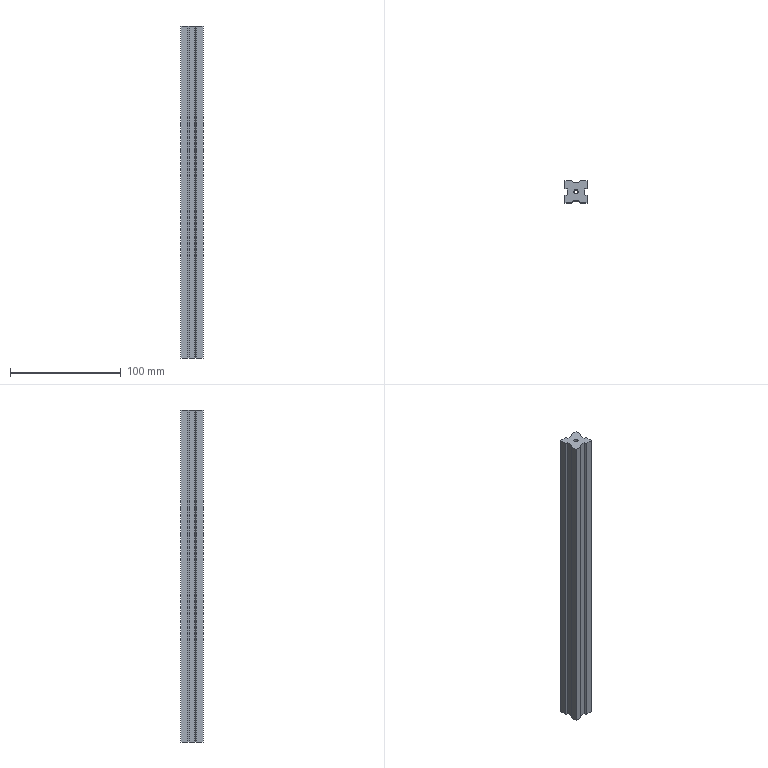Part | SolidWorks | features CirPattern 1, Extrusion 1, ICE 1 | 1 solid | 24 faces | box 20 x 20 x 300 mm | volume 101058 mm3 | plane 22 | cylinder 2 | commonest cylinder face diameters 3.889 x2
STEP:
#1=CARTESIAN_POINT('',(-1.944,0.,150.));
#2=VERTEX_POINT('',#1);
#3=CARTESIAN_POINT('',(1.944,0.,150.));
#4=VERTEX_POINT('',#3);
#5=CARTESIAN_POINT('',(0.,0.,150.));
#6=DIRECTION('',(0.,0.,1.));
#7=DIRECTION('',(1.,0.,0.));
#8=AXIS2_PLACEMENT_3D('',#5,#6,#7);
#9=CIRCLE('',#8,1.944);
#10=EDGE_CURVE('',#2,#4,#9,.T.);
#11=ORIENTED_EDGE('',*,*,#10,.T.);
#12=CARTESIAN_POINT('',(1.944,0.,-150.));
#13=VERTEX_POINT('',#12);
#14=CARTESIAN_POINT('',(1.944,0.,150.));
#15=DIRECTION('',(0.,0.,-1.));
#16=VECTOR('',#15,1000.);
#17=LINE('',#14,#16);
#18=EDGE_CURVE('',#4,#13,#17,.T.);
#19=ORIENTED_EDGE('',*,*,#18,.T.);
#20=CARTESIAN_POINT('',(-1.944,0.,-150.));
#21=VERTEX_POINT('',#20);
#22=CARTESIAN_POINT('',(0.,0.,-150.));
#23=DIRECTION('',(0.,0.,1.));
#24=DIRECTION('',(1.,0.,0.));
#25=AXIS2_PLACEMENT_3D('',#22,#23,#24);
#26=CIRCLE('',#25,1.944);
#27=EDGE_CURVE('',#21,#13,#26,.T.);
#28=ORIENTED_EDGE('',*,*,#27,.F.);
#29=CARTESIAN_POINT('',(-1.944,0.,150.));
#30=DIRECTION('',(0.,0.,-1.));
#31=VECTOR('',#30,1000.);
#32=LINE('',#29,#31);
#33=EDGE_CURVE('',#2,#21,#32,.T.);
#34=ORIENTED_EDGE('',*,*,#33,.F.);
#35=EDGE_LOOP('',(#11,#19,#28,#34));
#36=FACE_OUTER_BOUND('',#35,.T.);
#37=CARTESIAN_POINT('',(0.,0.,150.));
#38=DIRECTION('',(0.,0.,-1.));
#39=DIRECTION('',(-1.,0.,0.));
#40=AXIS2_PLACEMENT_3D('',#37,#38,#39);
#41=CYLINDRICAL_SURFACE('',#40,1.944);
#42=ADVANCED_FACE('',(#36),#41,.F.);
#43=CARTESIAN_POINT('',(-10.,3.694,150.));
#44=VERTEX_POINT('',#43);
#45=CARTESIAN_POINT('',(-10.,3.694,-150.));
#46=VERTEX_POINT('',#45);
#47=CARTESIAN_POINT('',(-10.,3.694,526.663));
#48=DIRECTION('',(0.,0.,-1.));
#49=VECTOR('',#48,1000.);
#50=LINE('',#47,#49);
#51=EDGE_CURVE('',#44,#46,#50,.T.);
#52=ORIENTED_EDGE('',*,*,#51,.F.);
#53=CARTESIAN_POINT('',(-10.,10.,150.));
#54=VERTEX_POINT('',#53);
#55=CARTESIAN_POINT('',(-10.,-10.,150.));
#56=DIRECTION('',(0.,-1.,0.));
#57=VECTOR('',#56,1000.);
#58=LINE('',#55,#57);
#59=EDGE_CURVE('',#54,#44,#58,.T.);
#60=ORIENTED_EDGE('',*,*,#59,.F.);
#61=CARTESIAN_POINT('',(-10.,10.,-150.));
#62=VERTEX_POINT('',#61);
#63=CARTESIAN_POINT('',(-10.,10.,150.));
#64=DIRECTION('',(0.,0.,-1.));
#65=VECTOR('',#64,1000.);
#66=LINE('',#63,#65);
#67=EDGE_CURVE('',#54,#62,#66,.T.);
#68=ORIENTED_EDGE('',*,*,#67,.T.);
#69=CARTESIAN_POINT('',(-10.,-10.,-150.));
#70=DIRECTION('',(0.,-1.,0.));
#71=VECTOR('',#70,1000.);
#72=LINE('',#69,#71);
#73=EDGE_CURVE('',#62,#46,#72,.T.);
#74=ORIENTED_EDGE('',*,*,#73,.T.);
#75=EDGE_LOOP('',(#52,#60,#68,#74));
#76=FACE_OUTER_BOUND('',#75,.T.);
#77=CARTESIAN_POINT('',(-10.,-10.,150.));
#78=DIRECTION('',(1.,0.,0.));
#79=DIRECTION('',(0.,0.,-1.));
#80=AXIS2_PLACEMENT_3D('',#77,#78,#79);
#81=PLANE('',#80);
#82=ADVANCED_FACE('',(#76),#81,.F.);
#83=ORIENTED_EDGE('',*,*,#10,.F.);
#84=CARTESIAN_POINT('',(0.,0.,150.));
#85=DIRECTION('',(0.,0.,1.));
#86=DIRECTION('',(1.,0.,0.));
#87=AXIS2_PLACEMENT_3D('',#84,#85,#86);
#88=CIRCLE('',#87,1.944);
#89=EDGE_CURVE('',#4,#2,#88,.T.);
#90=ORIENTED_EDGE('',*,*,#89,.F.);
#91=EDGE_LOOP('',(#83,#90));
#92=FACE_BOUND('',#91,.T.);
#93=CARTESIAN_POINT('',(-7.931,2.5,150.));
#94=VERTEX_POINT('',#93);
#95=CARTESIAN_POINT('',(-7.931,-2.5,150.));
#96=VERTEX_POINT('',#95);
#97=CARTESIAN_POINT('',(-7.931,0.,150.));
#98=DIRECTION('',(0.,-1.,0.));
#99=VECTOR('',#98,1000.);
#100=LINE('',#97,#99);
#101=EDGE_CURVE('',#94,#96,#100,.T.);
#102=ORIENTED_EDGE('',*,*,#101,.T.);
#103=CARTESIAN_POINT('',(-10.,-3.694,150.));
#104=VERTEX_POINT('',#103);
#105=CARTESIAN_POINT('',(-0.9003,1.559,150.));
#106=DIRECTION('',(-0.866,-0.5,0.));
#107=VECTOR('',#106,1000.);
#108=LINE('',#105,#107);
#109=EDGE_CURVE('',#96,#104,#108,.T.);
#110=ORIENTED_EDGE('',*,*,#109,.T.);
#111=CARTESIAN_POINT('',(-10.,-10.,150.));
#112=VERTEX_POINT('',#111);
#113=CARTESIAN_POINT('',(-10.,-10.,150.));
#114=DIRECTION('',(0.,-1.,0.));
#115=VECTOR('',#114,1000.);
#116=LINE('',#113,#115);
#117=EDGE_CURVE('',#104,#112,#116,.T.);
#118=ORIENTED_EDGE('',*,*,#117,.T.);
#119=CARTESIAN_POINT('',(-3.694,-10.,150.));
#120=VERTEX_POINT('',#119);
#121=CARTESIAN_POINT('',(10.,-10.,150.));
#122=DIRECTION('',(1.,0.,0.));
#123=VECTOR('',#122,1000.);
#124=LINE('',#121,#123);
#125=EDGE_CURVE('',#112,#120,#124,.T.);
#126=ORIENTED_EDGE('',*,*,#125,.T.);
#127=CARTESIAN_POINT('',(-2.5,-7.931,150.));
#128=VERTEX_POINT('',#127);
#129=CARTESIAN_POINT('',(1.559,-0.9003,150.));
#130=DIRECTION('',(0.5,0.866,0.));
#131=VECTOR('',#130,1000.);
#132=LINE('',#129,#131);
#133=EDGE_CURVE('',#120,#128,#132,.T.);
#134=ORIENTED_EDGE('',*,*,#133,.T.);
#135=CARTESIAN_POINT('',(2.5,-7.931,150.));
#136=VERTEX_POINT('',#135);
#137=CARTESIAN_POINT('',(0.,-7.931,150.));
#138=DIRECTION('',(1.,0.,0.));
#139=VECTOR('',#138,1000.);
#140=LINE('',#137,#139);
#141=EDGE_CURVE('',#128,#136,#140,.T.);
#142=ORIENTED_EDGE('',*,*,#141,.T.);
#143=CARTESIAN_POINT('',(3.694,-10.,150.));
#144=VERTEX_POINT('',#143);
#145=CARTESIAN_POINT('',(-1.559,-0.9003,150.));
#146=DIRECTION('',(0.5,-0.866,0.));
#147=VECTOR('',#146,1000.);
#148=LINE('',#145,#147);
#149=EDGE_CURVE('',#136,#144,#148,.T.);
#150=ORIENTED_EDGE('',*,*,#149,.T.);
#151=CARTESIAN_POINT('',(10.,-10.,150.));
#152=VERTEX_POINT('',#151);
#153=CARTESIAN_POINT('',(10.,-10.,150.));
#154=DIRECTION('',(1.,0.,0.));
#155=VECTOR('',#154,1000.);
#156=LINE('',#153,#155);
#157=EDGE_CURVE('',#144,#152,#156,.T.);
#158=ORIENTED_EDGE('',*,*,#157,.T.);
#159=CARTESIAN_POINT('',(10.,-3.694,150.));
#160=VERTEX_POINT('',#159);
#161=CARTESIAN_POINT('',(10.,-10.,150.));
#162=DIRECTION('',(0.,1.,0.));
#163=VECTOR('',#162,1000.);
#164=LINE('',#161,#163);
#165=EDGE_CURVE('',#152,#160,#164,.T.);
#166=ORIENTED_EDGE('',*,*,#165,.T.);
#167=CARTESIAN_POINT('',(7.931,-2.5,150.));
#168=VERTEX_POINT('',#167);
#169=CARTESIAN_POINT('',(0.9003,1.559,150.));
#170=DIRECTION('',(-0.866,0.5,0.));
#171=VECTOR('',#170,1000.);
#172=LINE('',#169,#171);
#173=EDGE_CURVE('',#160,#168,#172,.T.);
#174=ORIENTED_EDGE('',*,*,#173,.T.);
#175=CARTESIAN_POINT('',(7.931,2.5,150.));
#176=VERTEX_POINT('',#175);
#177=CARTESIAN_POINT('',(7.931,0.,150.));
#178=DIRECTION('',(0.,1.,0.));
#179=VECTOR('',#178,1000.);
#180=LINE('',#177,#179);
#181=EDGE_CURVE('',#168,#176,#180,.T.);
#182=ORIENTED_EDGE('',*,*,#181,.T.);
#183=CARTESIAN_POINT('',(10.,3.694,150.));
#184=VERTEX_POINT('',#183);
#185=CARTESIAN_POINT('',(0.9003,-1.559,150.));
#186=DIRECTION('',(0.866,0.5,0.));
#187=VECTOR('',#186,1000.);
#188=LINE('',#185,#187);
#189=EDGE_CURVE('',#176,#184,#188,.T.);
#190=ORIENTED_EDGE('',*,*,#189,.T.);
#191=CARTESIAN_POINT('',(10.,10.,150.));
#192=VERTEX_POINT('',#191);
#193=CARTESIAN_POINT('',(10.,-10.,150.));
#194=DIRECTION('',(0.,1.,0.));
#195=VECTOR('',#194,1000.);
#196=LINE('',#193,#195);
#197=EDGE_CURVE('',#184,#192,#196,.T.);
#198=ORIENTED_EDGE('',*,*,#197,.T.);
#199=CARTESIAN_POINT('',(3.694,10.,150.));
#200=VERTEX_POINT('',#199);
#201=CARTESIAN_POINT('',(10.,10.,150.));
#202=DIRECTION('',(-1.,0.,0.));
#203=VECTOR('',#202,1000.);
#204=LINE('',#201,#203);
#205=EDGE_CURVE('',#192,#200,#204,.T.);
#206=ORIENTED_EDGE('',*,*,#205,.T.);
#207=CARTESIAN_POINT('',(2.5,7.931,150.));
#208=VERTEX_POINT('',#207);
#209=CARTESIAN_POINT('',(-1.559,0.9003,150.));
#210=DIRECTION('',(-0.5,-0.866,0.));
#211=VECTOR('',#210,1000.);
#212=LINE('',#209,#211);
#213=EDGE_CURVE('',#200,#208,#212,.T.);
#214=ORIENTED_EDGE('',*,*,#213,.T.);
#215=CARTESIAN_POINT('',(-2.5,7.931,150.));
#216=VERTEX_POINT('',#215);
#217=CARTESIAN_POINT('',(0.,7.931,150.));
#218=DIRECTION('',(-1.,0.,0.));
#219=VECTOR('',#218,1000.);
#220=LINE('',#217,#219);
#221=EDGE_CURVE('',#208,#216,#220,.T.);
#222=ORIENTED_EDGE('',*,*,#221,.T.);
#223=CARTESIAN_POINT('',(-3.694,10.,150.));
#224=VERTEX_POINT('',#223);
#225=CARTESIAN_POINT('',(1.559,0.9003,150.));
#226=DIRECTION('',(-0.5,0.866,0.));
#227=VECTOR('',#226,1000.);
#228=LINE('',#225,#227);
#229=EDGE_CURVE('',#216,#224,#228,.T.);
#230=ORIENTED_EDGE('',*,*,#229,.T.);
#231=CARTESIAN_POINT('',(10.,10.,150.));
#232=DIRECTION('',(-1.,0.,0.));
#233=VECTOR('',#232,1000.);
#234=LINE('',#231,#233);
#235=EDGE_CURVE('',#224,#54,#234,.T.);
#236=ORIENTED_EDGE('',*,*,#235,.T.);
#237=ORIENTED_EDGE('',*,*,#59,.T.);
#238=CARTESIAN_POINT('',(-0.9003,-1.559,150.));
#239=DIRECTION('',(0.866,-0.5,0.));
#240=VECTOR('',#239,1000.);
#241=LINE('',#238,#240);
#242=EDGE_CURVE('',#44,#94,#241,.T.);
#243=ORIENTED_EDGE('',*,*,#242,.T.);
#244=EDGE_LOOP('',(#102,#110,#118,#126,#134,#142,#150,#158,#166,#174,#182,#190,#198,#206,#214,#222,#230,#236,#237,#243));
#245=FACE_OUTER_BOUND('',#244,.T.);
#246=CARTESIAN_POINT('',(0.,0.,150.));
#247=DIRECTION('',(0.,0.,1.));
#248=DIRECTION('',(1.,0.,0.));
#249=AXIS2_PLACEMENT_3D('',#246,#247,#248);
#250=PLANE('',#249);
#251=ADVANCED_FACE('',(#92,#245),#250,.T.);
#252=ORIENTED_EDGE('',*,*,#27,.T.);
#253=CARTESIAN_POINT('',(0.,0.,-150.));
#254=DIRECTION('',(0.,0.,1.));
#255=DIRECTION('',(1.,0.,0.));
#256=AXIS2_PLACEMENT_3D('',#253,#254,#255);
#257=CIRCLE('',#256,1.944);
#258=EDGE_CURVE('',#13,#21,#257,.T.);
#259=ORIENTED_EDGE('',*,*,#258,.T.);
#260=EDGE_LOOP('',(#252,#259));
#261=FACE_BOUND('',#260,.T.);
#262=CARTESIAN_POINT('',(-7.931,-2.5,-150.));
#263=VERTEX_POINT('',#262);
#264=CARTESIAN_POINT('',(-10.,-3.694,-150.));
#265=VERTEX_POINT('',#264);
#266=CARTESIAN_POINT('',(-0.9003,1.559,-150.));
#267=DIRECTION('',(-0.866,-0.5,0.));
#268=VECTOR('',#267,1000.);
#269=LINE('',#266,#268);
#270=EDGE_CURVE('',#263,#265,#269,.T.);
#271=ORIENTED_EDGE('',*,*,#270,.F.);
#272=CARTESIAN_POINT('',(-7.931,2.5,-150.));
#273=VERTEX_POINT('',#272);
#274=CARTESIAN_POINT('',(-7.931,0.,-150.));
#275=DIRECTION('',(0.,-1.,0.));
#276=VECTOR('',#275,1000.);
#277=LINE('',#274,#276);
#278=EDGE_CURVE('',#273,#263,#277,.T.);
#279=ORIENTED_EDGE('',*,*,#278,.F.);
#280=CARTESIAN_POINT('',(-0.9003,-1.559,-150.));
#281=DIRECTION('',(0.866,-0.5,0.));
#282=VECTOR('',#281,1000.);
#283=LINE('',#280,#282);
#284=EDGE_CURVE('',#46,#273,#283,.T.);
#285=ORIENTED_EDGE('',*,*,#284,.F.);
#286=ORIENTED_EDGE('',*,*,#73,.F.);
#287=CARTESIAN_POINT('',(-3.694,10.,-150.));
#288=VERTEX_POINT('',#287);
#289=CARTESIAN_POINT('',(10.,10.,-150.));
#290=DIRECTION('',(-1.,0.,0.));
#291=VECTOR('',#290,1000.);
#292=LINE('',#289,#291);
#293=EDGE_CURVE('',#288,#62,#292,.T.);
#294=ORIENTED_EDGE('',*,*,#293,.F.);
#295=CARTESIAN_POINT('',(-2.5,7.931,-150.));
#296=VERTEX_POINT('',#295);
#297=CARTESIAN_POINT('',(1.559,0.9003,-150.));
#298=DIRECTION('',(-0.5,0.866,0.));
#299=VECTOR('',#298,1000.);
#300=LINE('',#297,#299);
#301=EDGE_CURVE('',#296,#288,#300,.T.);
#302=ORIENTED_EDGE('',*,*,#301,.F.);
#303=CARTESIAN_POINT('',(2.5,7.931,-150.));
#304=VERTEX_POINT('',#303);
#305=CARTESIAN_POINT('',(0.,7.931,-150.));
#306=DIRECTION('',(-1.,0.,0.));
#307=VECTOR('',#306,1000.);
#308=LINE('',#305,#307);
#309=EDGE_CURVE('',#304,#296,#308,.T.);
#310=ORIENTED_EDGE('',*,*,#309,.F.);
#311=CARTESIAN_POINT('',(3.694,10.,-150.));
#312=VERTEX_POINT('',#311);
#313=CARTESIAN_POINT('',(-1.559,0.9003,-150.));
#314=DIRECTION('',(-0.5,-0.866,0.));
#315=VECTOR('',#314,1000.);
#316=LINE('',#313,#315);
#317=EDGE_CURVE('',#312,#304,#316,.T.);
#318=ORIENTED_EDGE('',*,*,#317,.F.);
#319=CARTESIAN_POINT('',(10.,10.,-150.));
#320=VERTEX_POINT('',#319);
#321=CARTESIAN_POINT('',(10.,10.,-150.));
#322=DIRECTION('',(-1.,0.,0.));
#323=VECTOR('',#322,1000.);
#324=LINE('',#321,#323);
#325=EDGE_CURVE('',#320,#312,#324,.T.);
#326=ORIENTED_EDGE('',*,*,#325,.F.);
#327=CARTESIAN_POINT('',(10.,3.694,-150.));
#328=VERTEX_POINT('',#327);
#329=CARTESIAN_POINT('',(10.,-10.,-150.));
#330=DIRECTION('',(0.,1.,0.));
#331=VECTOR('',#330,1000.);
#332=LINE('',#329,#331);
#333=EDGE_CURVE('',#328,#320,#332,.T.);
#334=ORIENTED_EDGE('',*,*,#333,.F.);
#335=CARTESIAN_POINT('',(7.931,2.5,-150.));
#336=VERTEX_POINT('',#335);
#337=CARTESIAN_POINT('',(0.9003,-1.559,-150.));
#338=DIRECTION('',(0.866,0.5,0.));
#339=VECTOR('',#338,1000.);
#340=LINE('',#337,#339);
#341=EDGE_CURVE('',#336,#328,#340,.T.);
#342=ORIENTED_EDGE('',*,*,#341,.F.);
#343=CARTESIAN_POINT('',(7.931,-2.5,-150.));
#344=VERTEX_POINT('',#343);
#345=CARTESIAN_POINT('',(7.931,0.,-150.));
#346=DIRECTION('',(0.,1.,0.));
#347=VECTOR('',#346,1000.);
#348=LINE('',#345,#347);
#349=EDGE_CURVE('',#344,#336,#348,.T.);
#350=ORIENTED_EDGE('',*,*,#349,.F.);
#351=CARTESIAN_POINT('',(10.,-3.694,-150.));
#352=VERTEX_POINT('',#351);
#353=CARTESIAN_POINT('',(0.9003,1.559,-150.));
#354=DIRECTION('',(-0.866,0.5,0.));
#355=VECTOR('',#354,1000.);
#356=LINE('',#353,#355);
#357=EDGE_CURVE('',#352,#344,#356,.T.);
#358=ORIENTED_EDGE('',*,*,#357,.F.);
#359=CARTESIAN_POINT('',(10.,-10.,-150.));
#360=VERTEX_POINT('',#359);
#361=CARTESIAN_POINT('',(10.,-10.,-150.));
#362=DIRECTION('',(0.,1.,0.));
#363=VECTOR('',#362,1000.);
#364=LINE('',#361,#363);
#365=EDGE_CURVE('',#360,#352,#364,.T.);
#366=ORIENTED_EDGE('',*,*,#365,.F.);
#367=CARTESIAN_POINT('',(3.694,-10.,-150.));
#368=VERTEX_POINT('',#367);
#369=CARTESIAN_POINT('',(10.,-10.,-150.));
#370=DIRECTION('',(1.,0.,0.));
#371=VECTOR('',#370,1000.);
#372=LINE('',#369,#371);
#373=EDGE_CURVE('',#368,#360,#372,.T.);
#374=ORIENTED_EDGE('',*,*,#373,.F.);
#375=CARTESIAN_POINT('',(2.5,-7.931,-150.));
#376=VERTEX_POINT('',#375);
#377=CARTESIAN_POINT('',(-1.559,-0.9003,-150.));
#378=DIRECTION('',(0.5,-0.866,0.));
#379=VECTOR('',#378,1000.);
#380=LINE('',#377,#379);
#381=EDGE_CURVE('',#376,#368,#380,.T.);
#382=ORIENTED_EDGE('',*,*,#381,.F.);
#383=CARTESIAN_POINT('',(-2.5,-7.931,-150.));
#384=VERTEX_POINT('',#383);
#385=CARTESIAN_POINT('',(0.,-7.931,-150.));
#386=DIRECTION('',(1.,0.,0.));
#387=VECTOR('',#386,1000.);
#388=LINE('',#385,#387);
#389=EDGE_CURVE('',#384,#376,#388,.T.);
#390=ORIENTED_EDGE('',*,*,#389,.F.);
#391=CARTESIAN_POINT('',(-3.694,-10.,-150.));
#392=VERTEX_POINT('',#391);
#393=CARTESIAN_POINT('',(1.559,-0.9003,-150.));
#394=DIRECTION('',(0.5,0.866,0.));
#395=VECTOR('',#394,1000.);
#396=LINE('',#393,#395);
#397=EDGE_CURVE('',#392,#384,#396,.T.);
#398=ORIENTED_EDGE('',*,*,#397,.F.);
#399=CARTESIAN_POINT('',(-10.,-10.,-150.));
#400=VERTEX_POINT('',#399);
#401=CARTESIAN_POINT('',(10.,-10.,-150.));
#402=DIRECTION('',(1.,0.,0.));
#403=VECTOR('',#402,1000.);
#404=LINE('',#401,#403);
#405=EDGE_CURVE('',#400,#392,#404,.T.);
#406=ORIENTED_EDGE('',*,*,#405,.F.);
#407=CARTESIAN_POINT('',(-10.,-10.,-150.));
#408=DIRECTION('',(0.,-1.,0.));
#409=VECTOR('',#408,1000.);
#410=LINE('',#407,#409);
#411=EDGE_CURVE('',#265,#400,#410,.T.);
#412=ORIENTED_EDGE('',*,*,#411,.F.);
#413=EDGE_LOOP('',(#271,#279,#285,#286,#294,#302,#310,#318,#326,#334,#342,#350,#358,#366,#374,#382,#390,#398,#406,#412));
#414=FACE_OUTER_BOUND('',#413,.T.);
#415=CARTESIAN_POINT('',(0.,0.,-150.));
#416=DIRECTION('',(0.,0.,1.));
#417=DIRECTION('',(1.,0.,0.));
#418=AXIS2_PLACEMENT_3D('',#415,#416,#417);
#419=PLANE('',#418);
#420=ADVANCED_FACE('',(#261,#414),#419,.F.);
#421=CARTESIAN_POINT('',(-3.694,-10.,526.663));
#422=DIRECTION('',(0.,0.,-1.));
#423=VECTOR('',#422,1000.);
#424=LINE('',#421,#423);
#425=EDGE_CURVE('',#120,#392,#424,.T.);
#426=ORIENTED_EDGE('',*,*,#425,.F.);
#427=ORIENTED_EDGE('',*,*,#125,.F.);
#428=CARTESIAN_POINT('',(-10.,-10.,150.));
#429=DIRECTION('',(0.,0.,-1.));
#430=VECTOR('',#429,1000.);
#431=LINE('',#428,#430);
#432=EDGE_CURVE('',#112,#400,#431,.T.);
#433=ORIENTED_EDGE('',*,*,#432,.T.);
#434=ORIENTED_EDGE('',*,*,#405,.T.);
#435=EDGE_LOOP('',(#426,#427,#433,#434));
#436=FACE_OUTER_BOUND('',#435,.T.);
#437=CARTESIAN_POINT('',(10.,-10.,150.));
#438=DIRECTION('',(0.,1.,0.));
#439=DIRECTION('',(-1.,0.,0.));
#440=AXIS2_PLACEMENT_3D('',#437,#438,#439);
#441=PLANE('',#440);
#442=ADVANCED_FACE('',(#436),#441,.F.);
#443=CARTESIAN_POINT('',(10.,-3.694,526.663));
#444=DIRECTION('',(0.,0.,-1.));
#445=VECTOR('',#444,1000.);
#446=LINE('',#443,#445);
#447=EDGE_CURVE('',#160,#352,#446,.T.);
#448=ORIENTED_EDGE('',*,*,#447,.F.);
#449=ORIENTED_EDGE('',*,*,#165,.F.);
#450=CARTESIAN_POINT('',(10.,-10.,150.));
#451=DIRECTION('',(0.,0.,-1.));
#452=VECTOR('',#451,1000.);
#453=LINE('',#450,#452);
#454=EDGE_CURVE('',#152,#360,#453,.T.);
#455=ORIENTED_EDGE('',*,*,#454,.T.);
#456=ORIENTED_EDGE('',*,*,#365,.T.);
#457=EDGE_LOOP('',(#448,#449,#455,#456));
#458=FACE_OUTER_BOUND('',#457,.T.);
#459=CARTESIAN_POINT('',(10.,-10.,150.));
#460=DIRECTION('',(-1.,0.,0.));
#461=DIRECTION('',(0.,0.,1.));
#462=AXIS2_PLACEMENT_3D('',#459,#460,#461);
#463=PLANE('',#462);
#464=ADVANCED_FACE('',(#458),#463,.F.);
#465=CARTESIAN_POINT('',(3.694,10.,526.663));
#466=DIRECTION('',(0.,0.,-1.));
#467=VECTOR('',#466,1000.);
#468=LINE('',#465,#467);
#469=EDGE_CURVE('',#200,#312,#468,.T.);
#470=ORIENTED_EDGE('',*,*,#469,.F.);
#471=ORIENTED_EDGE('',*,*,#205,.F.);
#472=CARTESIAN_POINT('',(10.,10.,150.));
#473=DIRECTION('',(0.,0.,-1.));
#474=VECTOR('',#473,1000.);
#475=LINE('',#472,#474);
#476=EDGE_CURVE('',#192,#320,#475,.T.);
#477=ORIENTED_EDGE('',*,*,#476,.T.);
#478=ORIENTED_EDGE('',*,*,#325,.T.);
#479=EDGE_LOOP('',(#470,#471,#477,#478));
#480=FACE_OUTER_BOUND('',#479,.T.);
#481=CARTESIAN_POINT('',(10.,10.,150.));
#482=DIRECTION('',(0.,-1.,0.));
#483=DIRECTION('',(1.,0.,0.));
#484=AXIS2_PLACEMENT_3D('',#481,#482,#483);
#485=PLANE('',#484);
#486=ADVANCED_FACE('',(#480),#485,.F.);
#487=ORIENTED_EDGE('',*,*,#117,.F.);
#488=CARTESIAN_POINT('',(-10.,-3.694,526.663));
#489=DIRECTION('',(0.,0.,-1.));
#490=VECTOR('',#489,1000.);
#491=LINE('',#488,#490);
#492=EDGE_CURVE('',#104,#265,#491,.T.);
#493=ORIENTED_EDGE('',*,*,#492,.T.);
#494=ORIENTED_EDGE('',*,*,#411,.T.);
#495=ORIENTED_EDGE('',*,*,#432,.F.);
#496=EDGE_LOOP('',(#487,#493,#494,#495));
#497=FACE_OUTER_BOUND('',#496,.T.);
#498=CARTESIAN_POINT('',(-10.,-10.,150.));
#499=DIRECTION('',(1.,0.,0.));
#500=DIRECTION('',(0.,0.,-1.));
#501=AXIS2_PLACEMENT_3D('',#498,#499,#500);
#502=PLANE('',#501);
#503=ADVANCED_FACE('',(#497),#502,.F.);
#504=ORIENTED_EDGE('',*,*,#157,.F.);
#505=CARTESIAN_POINT('',(3.694,-10.,526.663));
#506=DIRECTION('',(0.,0.,-1.));
#507=VECTOR('',#506,1000.);
#508=LINE('',#505,#507);
#509=EDGE_CURVE('',#144,#368,#508,.T.);
#510=ORIENTED_EDGE('',*,*,#509,.T.);
#511=ORIENTED_EDGE('',*,*,#373,.T.);
#512=ORIENTED_EDGE('',*,*,#454,.F.);
#513=EDGE_LOOP('',(#504,#510,#511,#512));
#514=FACE_OUTER_BOUND('',#513,.T.);
#515=CARTESIAN_POINT('',(10.,-10.,150.));
#516=DIRECTION('',(0.,1.,0.));
#517=DIRECTION('',(-1.,0.,0.));
#518=AXIS2_PLACEMENT_3D('',#515,#516,#517);
#519=PLANE('',#518);
#520=ADVANCED_FACE('',(#514),#519,.F.);
#521=ORIENTED_EDGE('',*,*,#197,.F.);
#522=CARTESIAN_POINT('',(10.,3.694,526.663));
#523=DIRECTION('',(0.,0.,-1.));
#524=VECTOR('',#523,1000.);
#525=LINE('',#522,#524);
#526=EDGE_CURVE('',#184,#328,#525,.T.);
#527=ORIENTED_EDGE('',*,*,#526,.T.);
#528=ORIENTED_EDGE('',*,*,#333,.T.);
#529=ORIENTED_EDGE('',*,*,#476,.F.);
#530=EDGE_LOOP('',(#521,#527,#528,#529));
#531=FACE_OUTER_BOUND('',#530,.T.);
#532=CARTESIAN_POINT('',(10.,-10.,150.));
#533=DIRECTION('',(-1.,0.,0.));
#534=DIRECTION('',(0.,0.,1.));
#535=AXIS2_PLACEMENT_3D('',#532,#533,#534);
#536=PLANE('',#535);
#537=ADVANCED_FACE('',(#531),#536,.F.);
#538=ORIENTED_EDGE('',*,*,#235,.F.);
#539=CARTESIAN_POINT('',(-3.694,10.,526.663));
#540=DIRECTION('',(0.,0.,-1.));
#541=VECTOR('',#540,1000.);
#542=LINE('',#539,#541);
#543=EDGE_CURVE('',#224,#288,#542,.T.);
#544=ORIENTED_EDGE('',*,*,#543,.T.);
#545=ORIENTED_EDGE('',*,*,#293,.T.);
#546=ORIENTED_EDGE('',*,*,#67,.F.);
#547=EDGE_LOOP('',(#538,#544,#545,#546));
#548=FACE_OUTER_BOUND('',#547,.T.);
#549=CARTESIAN_POINT('',(10.,10.,150.));
#550=DIRECTION('',(0.,-1.,0.));
#551=DIRECTION('',(1.,0.,0.));
#552=AXIS2_PLACEMENT_3D('',#549,#550,#551);
#553=PLANE('',#552);
#554=ADVANCED_FACE('',(#548),#553,.F.);
#555=ORIENTED_EDGE('',*,*,#18,.F.);
#556=ORIENTED_EDGE('',*,*,#89,.T.);
#557=ORIENTED_EDGE('',*,*,#33,.T.);
#558=ORIENTED_EDGE('',*,*,#258,.F.);
#559=EDGE_LOOP('',(#555,#556,#557,#558));
#560=FACE_OUTER_BOUND('',#559,.T.);
#561=CARTESIAN_POINT('',(0.,0.,150.));
#562=DIRECTION('',(0.,0.,-1.));
#563=DIRECTION('',(-1.,0.,0.));
#564=AXIS2_PLACEMENT_3D('',#561,#562,#563);
#565=CYLINDRICAL_SURFACE('',#564,1.944);
#566=ADVANCED_FACE('',(#560),#565,.F.);
#567=ORIENTED_EDGE('',*,*,#229,.F.);
#568=CARTESIAN_POINT('',(-2.5,7.931,526.663));
#569=DIRECTION('',(0.,0.,-1.));
#570=VECTOR('',#569,1000.);
#571=LINE('',#568,#570);
#572=EDGE_CURVE('',#216,#296,#571,.T.);
#573=ORIENTED_EDGE('',*,*,#572,.T.);
#574=ORIENTED_EDGE('',*,*,#301,.T.);
#575=ORIENTED_EDGE('',*,*,#543,.F.);
#576=EDGE_LOOP('',(#567,#573,#574,#575));
#577=FACE_OUTER_BOUND('',#576,.T.);
#578=CARTESIAN_POINT('',(-3.694,10.,526.663));
#579=DIRECTION('',(0.866,0.5,0.));
#580=DIRECTION('',(-0.5,0.866,0.));
#581=AXIS2_PLACEMENT_3D('',#578,#579,#580);
#582=PLANE('',#581);
#583=ADVANCED_FACE('',(#577),#582,.T.);
#584=ORIENTED_EDGE('',*,*,#221,.F.);
#585=CARTESIAN_POINT('',(2.5,7.931,526.663));
#586=DIRECTION('',(0.,0.,-1.));
#587=VECTOR('',#586,1000.);
#588=LINE('',#585,#587);
#589=EDGE_CURVE('',#208,#304,#588,.T.);
#590=ORIENTED_EDGE('',*,*,#589,.T.);
#591=ORIENTED_EDGE('',*,*,#309,.T.);
#592=ORIENTED_EDGE('',*,*,#572,.F.);
#593=EDGE_LOOP('',(#584,#590,#591,#592));
#594=FACE_OUTER_BOUND('',#593,.T.);
#595=CARTESIAN_POINT('',(-2.5,7.931,526.663));
#596=DIRECTION('',(0.,1.,0.));
#597=DIRECTION('',(0.,0.,1.));
#598=AXIS2_PLACEMENT_3D('',#595,#596,#597);
#599=PLANE('',#598);
#600=ADVANCED_FACE('',(#594),#599,.T.);
#601=ORIENTED_EDGE('',*,*,#213,.F.);
#602=ORIENTED_EDGE('',*,*,#469,.T.);
#603=ORIENTED_EDGE('',*,*,#317,.T.);
#604=ORIENTED_EDGE('',*,*,#589,.F.);
#605=EDGE_LOOP('',(#601,#602,#603,#604));
#606=FACE_OUTER_BOUND('',#605,.T.);
#607=CARTESIAN_POINT('',(2.5,7.931,526.663));
#608=DIRECTION('',(-0.866,0.5,0.));
#609=DIRECTION('',(-0.5,-0.866,0.));
#610=AXIS2_PLACEMENT_3D('',#607,#608,#609);
#611=PLANE('',#610);
#612=ADVANCED_FACE('',(#606),#611,.T.);
#613=ORIENTED_EDGE('',*,*,#189,.F.);
#614=CARTESIAN_POINT('',(7.931,2.5,526.663));
#615=DIRECTION('',(0.,0.,-1.));
#616=VECTOR('',#615,1000.);
#617=LINE('',#614,#616);
#618=EDGE_CURVE('',#176,#336,#617,.T.);
#619=ORIENTED_EDGE('',*,*,#618,.T.);
#620=ORIENTED_EDGE('',*,*,#341,.T.);
#621=ORIENTED_EDGE('',*,*,#526,.F.);
#622=EDGE_LOOP('',(#613,#619,#620,#621));
#623=FACE_OUTER_BOUND('',#622,.T.);
#624=CARTESIAN_POINT('',(10.,3.694,526.663));
#625=DIRECTION('',(0.5,-0.866,0.));
#626=DIRECTION('',(0.866,0.5,0.));
#627=AXIS2_PLACEMENT_3D('',#624,#625,#626);
#628=PLANE('',#627);
#629=ADVANCED_FACE('',(#623),#628,.T.);
#630=ORIENTED_EDGE('',*,*,#181,.F.);
#631=CARTESIAN_POINT('',(7.931,-2.5,526.663));
#632=DIRECTION('',(0.,0.,-1.));
#633=VECTOR('',#632,1000.);
#634=LINE('',#631,#633);
#635=EDGE_CURVE('',#168,#344,#634,.T.);
#636=ORIENTED_EDGE('',*,*,#635,.T.);
#637=ORIENTED_EDGE('',*,*,#349,.T.);
#638=ORIENTED_EDGE('',*,*,#618,.F.);
#639=EDGE_LOOP('',(#630,#636,#637,#638));
#640=FACE_OUTER_BOUND('',#639,.T.);
#641=CARTESIAN_POINT('',(7.931,2.5,526.663));
#642=DIRECTION('',(1.,0.,0.));
#643=DIRECTION('',(0.,1.,0.));
#644=AXIS2_PLACEMENT_3D('',#641,#642,#643);
#645=PLANE('',#644);
#646=ADVANCED_FACE('',(#640),#645,.T.);
#647=ORIENTED_EDGE('',*,*,#173,.F.);
#648=ORIENTED_EDGE('',*,*,#447,.T.);
#649=ORIENTED_EDGE('',*,*,#357,.T.);
#650=ORIENTED_EDGE('',*,*,#635,.F.);
#651=EDGE_LOOP('',(#647,#648,#649,#650));
#652=FACE_OUTER_BOUND('',#651,.T.);
#653=CARTESIAN_POINT('',(7.931,-2.5,526.663));
#654=DIRECTION('',(0.5,0.866,0.));
#655=DIRECTION('',(-0.866,0.5,0.));
#656=AXIS2_PLACEMENT_3D('',#653,#654,#655);
#657=PLANE('',#656);
#658=ADVANCED_FACE('',(#652),#657,.T.);
#659=ORIENTED_EDGE('',*,*,#149,.F.);
#660=CARTESIAN_POINT('',(2.5,-7.931,526.663));
#661=DIRECTION('',(0.,0.,-1.));
#662=VECTOR('',#661,1000.);
#663=LINE('',#660,#662);
#664=EDGE_CURVE('',#136,#376,#663,.T.);
#665=ORIENTED_EDGE('',*,*,#664,.T.);
#666=ORIENTED_EDGE('',*,*,#381,.T.);
#667=ORIENTED_EDGE('',*,*,#509,.F.);
#668=EDGE_LOOP('',(#659,#665,#666,#667));
#669=FACE_OUTER_BOUND('',#668,.T.);
#670=CARTESIAN_POINT('',(3.694,-10.,526.663));
#671=DIRECTION('',(-0.866,-0.5,0.));
#672=DIRECTION('',(0.5,-0.866,0.));
#673=AXIS2_PLACEMENT_3D('',#670,#671,#672);
#674=PLANE('',#673);
#675=ADVANCED_FACE('',(#669),#674,.T.);
#676=ORIENTED_EDGE('',*,*,#141,.F.);
#677=CARTESIAN_POINT('',(-2.5,-7.931,526.663));
#678=DIRECTION('',(0.,0.,-1.));
#679=VECTOR('',#678,1000.);
#680=LINE('',#677,#679);
#681=EDGE_CURVE('',#128,#384,#680,.T.);
#682=ORIENTED_EDGE('',*,*,#681,.T.);
#683=ORIENTED_EDGE('',*,*,#389,.T.);
#684=ORIENTED_EDGE('',*,*,#664,.F.);
#685=EDGE_LOOP('',(#676,#682,#683,#684));
#686=FACE_OUTER_BOUND('',#685,.T.);
#687=CARTESIAN_POINT('',(2.5,-7.931,526.663));
#688=DIRECTION('',(0.,-1.,0.));
#689=DIRECTION('',(0.,0.,-1.));
#690=AXIS2_PLACEMENT_3D('',#687,#688,#689);
#691=PLANE('',#690);
#692=ADVANCED_FACE('',(#686),#691,.T.);
#693=ORIENTED_EDGE('',*,*,#133,.F.);
#694=ORIENTED_EDGE('',*,*,#425,.T.);
#695=ORIENTED_EDGE('',*,*,#397,.T.);
#696=ORIENTED_EDGE('',*,*,#681,.F.);
#697=EDGE_LOOP('',(#693,#694,#695,#696));
#698=FACE_OUTER_BOUND('',#697,.T.);
#699=CARTESIAN_POINT('',(-2.5,-7.931,526.663));
#700=DIRECTION('',(0.866,-0.5,0.));
#701=DIRECTION('',(0.5,0.866,0.));
#702=AXIS2_PLACEMENT_3D('',#699,#700,#701);
#703=PLANE('',#702);
#704=ADVANCED_FACE('',(#698),#703,.T.);
#705=ORIENTED_EDGE('',*,*,#109,.F.);
#706=CARTESIAN_POINT('',(-7.931,-2.5,526.663));
#707=DIRECTION('',(0.,0.,-1.));
#708=VECTOR('',#707,1000.);
#709=LINE('',#706,#708);
#710=EDGE_CURVE('',#96,#263,#709,.T.);
#711=ORIENTED_EDGE('',*,*,#710,.T.);
#712=ORIENTED_EDGE('',*,*,#270,.T.);
#713=ORIENTED_EDGE('',*,*,#492,.F.);
#714=EDGE_LOOP('',(#705,#711,#712,#713));
#715=FACE_OUTER_BOUND('',#714,.T.);
#716=CARTESIAN_POINT('',(-10.,-3.694,526.663));
#717=DIRECTION('',(-0.5,0.866,0.));
#718=DIRECTION('',(-0.866,-0.5,0.));
#719=AXIS2_PLACEMENT_3D('',#716,#717,#718);
#720=PLANE('',#719);
#721=ADVANCED_FACE('',(#715),#720,.T.);
#722=ORIENTED_EDGE('',*,*,#101,.F.);
#723=CARTESIAN_POINT('',(-7.931,2.5,526.663));
#724=DIRECTION('',(0.,0.,-1.));
#725=VECTOR('',#724,1000.);
#726=LINE('',#723,#725);
#727=EDGE_CURVE('',#94,#273,#726,.T.);
#728=ORIENTED_EDGE('',*,*,#727,.T.);
#729=ORIENTED_EDGE('',*,*,#278,.T.);
#730=ORIENTED_EDGE('',*,*,#710,.F.);
#731=EDGE_LOOP('',(#722,#728,#729,#730));
#732=FACE_OUTER_BOUND('',#731,.T.);
#733=CARTESIAN_POINT('',(-7.931,-2.5,526.663));
#734=DIRECTION('',(-1.,0.,0.));
#735=DIRECTION('',(0.,-1.,0.));
#736=AXIS2_PLACEMENT_3D('',#733,#734,#735);
#737=PLANE('',#736);
#738=ADVANCED_FACE('',(#732),#737,.T.);
#739=ORIENTED_EDGE('',*,*,#242,.F.);
#740=ORIENTED_EDGE('',*,*,#51,.T.);
#741=ORIENTED_EDGE('',*,*,#284,.T.);
#742=ORIENTED_EDGE('',*,*,#727,.F.);
#743=EDGE_LOOP('',(#739,#740,#741,#742));
#744=FACE_OUTER_BOUND('',#743,.T.);
#745=CARTESIAN_POINT('',(-7.931,2.5,526.663));
#746=DIRECTION('',(-0.5,-0.866,0.));
#747=DIRECTION('',(0.866,-0.5,0.));
#748=AXIS2_PLACEMENT_3D('',#745,#746,#747);
#749=PLANE('',#748);
#750=ADVANCED_FACE('',(#744),#749,.T.);
#751=CLOSED_SHELL('',(#42,#82,#251,#420,#442,#464,#486,#503,#520,#537,#554,#566,#583,#600,#612,#629,#646,#658,#675,#692,#704,#721,#738,#750));
#752=MANIFOLD_SOLID_BREP('',#751);
#753=CARTESIAN_POINT('',(0.,0.,0.));
#754=DIRECTION('',(0.,0.,1.));
#755=DIRECTION('',(1.,0.,0.));
#756=AXIS2_PLACEMENT_3D('',#753,#754,#755);
#757=(LENGTH_UNIT()NAMED_UNIT(*)SI_UNIT(.MILLI.,.METRE.));
#758=UNCERTAINTY_MEASURE_WITH_UNIT(LENGTH_MEASURE(0.00001),#757,'','');
#759=(NAMED_UNIT(*)PLANE_ANGLE_UNIT()SI_UNIT($,.RADIAN.));
#760=(NAMED_UNIT(*)SI_UNIT($,.STERADIAN.)SOLID_ANGLE_UNIT());
#761=(GEOMETRIC_REPRESENTATION_CONTEXT(3)GLOBAL_UNCERTAINTY_ASSIGNED_CONTEXT((#758))GLOBAL_UNIT_ASSIGNED_CONTEXT((#757,#759,#760))REPRESENTATION_CONTEXT('',''));
#762=ADVANCED_BREP_SHAPE_REPRESENTATION('',(#752,#756),#761);